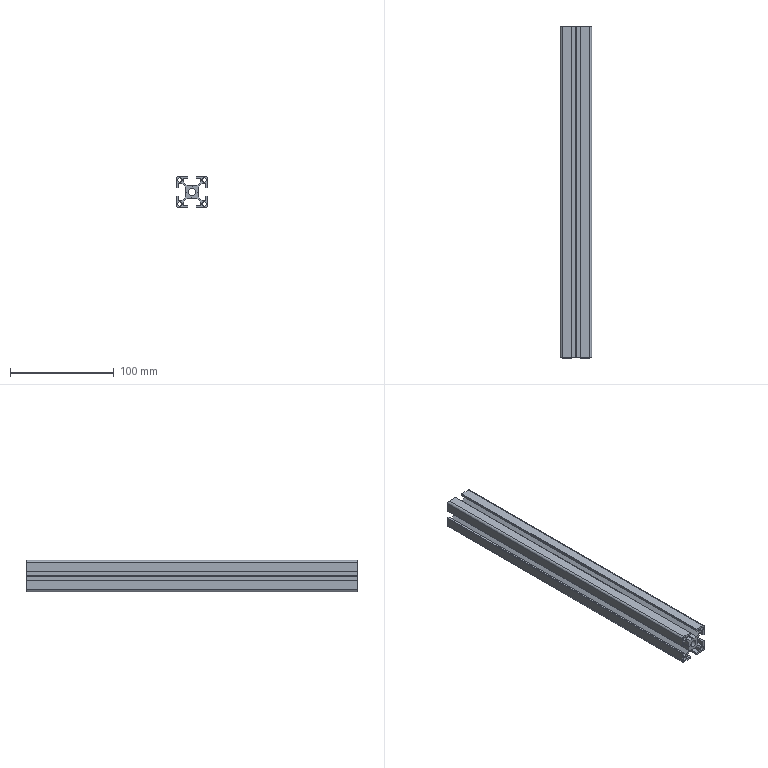Part | STEP file | ASND-0110-1-3 | 1 solid | 80 faces | box 30 x 320 x 30 mm | volume 106163 mm3 | plane 58 | cylinder 22 | commonest cylinder face diameters 0.6 x8 4.2 x8 4 x4 6.8 x2